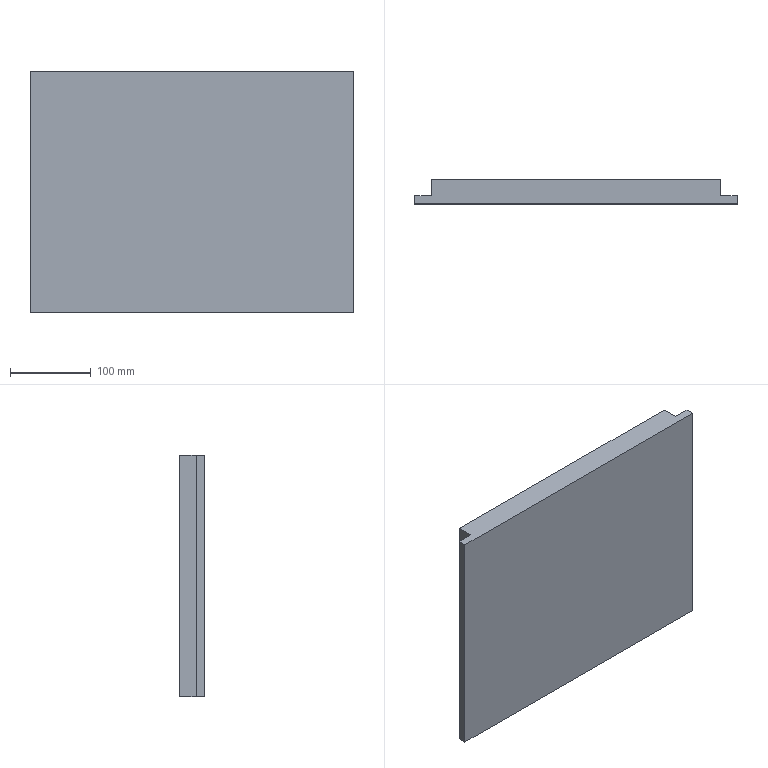Part | STEP file | PN_0004 jig | 1 solid | 77 faces | box 400 x 30 x 300 mm | volume 3171570 mm3 | plane 75 | spline 2